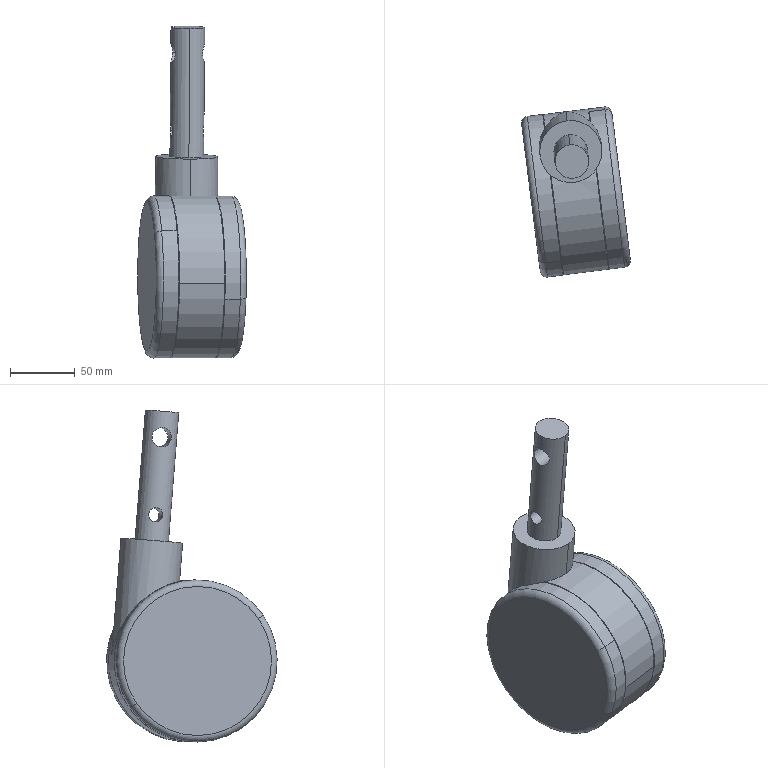Part | SolidWorks | features BaseBody 3 | 3 solids | 30 faces | box 83.862 x 131.58 x 256.05 mm | volume 967710 mm3 | cylinder 18 | plane 8 | torus 4 | commonest cylinder face diameters 125 x10 11 x2 15 x2 26 x2 48 x2